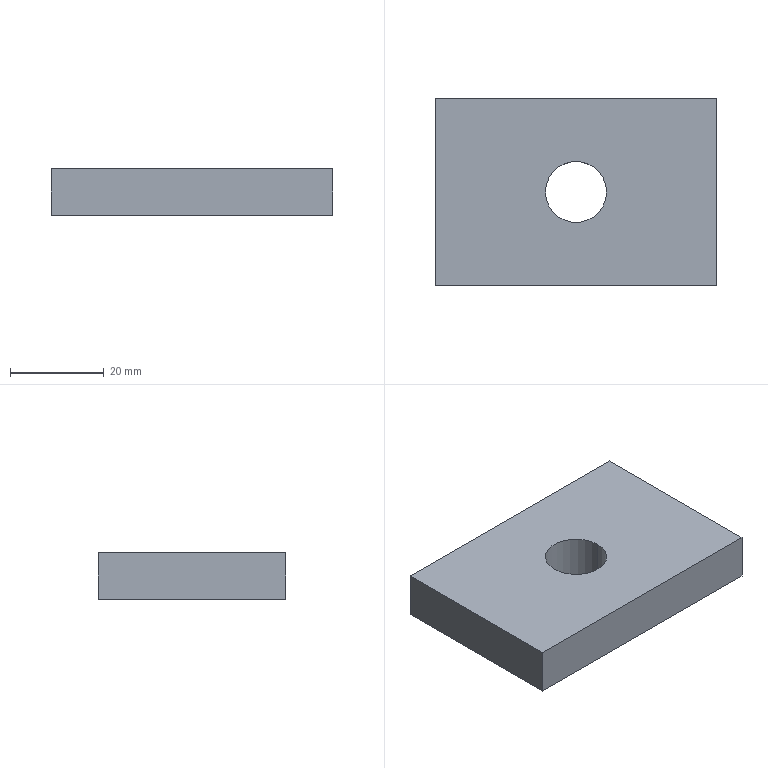Part | SolidWorks | features BaseBody 1 | 1 solid | 8 faces | box 60 x 40 x 10 mm | volume 22673 mm3 | plane 6 | cylinder 2 | commonest cylinder face diameters 13 x2
STEP:
#1=CARTESIAN_POINT('',(6.5,0.,0.));
#2=VERTEX_POINT('',#1);
#3=CARTESIAN_POINT('',(-6.5,0.,0.));
#4=VERTEX_POINT('',#3);
#5=CARTESIAN_POINT('',(0.,0.,0.));
#6=DIRECTION('',(0.,0.,-1.));
#7=DIRECTION('',(1.,0.,0.));
#8=AXIS2_PLACEMENT_3D('',#5,#6,#7);
#9=CIRCLE('',#8,6.5);
#10=EDGE_CURVE('',#2,#4,#9,.T.);
#11=ORIENTED_EDGE('',*,*,#10,.T.);
#12=CARTESIAN_POINT('',(-6.5,0.,10.));
#13=VERTEX_POINT('',#12);
#14=CARTESIAN_POINT('',(-6.5,0.,0.));
#15=DIRECTION('',(0.,0.,1.));
#16=VECTOR('',#15,1000.);
#17=LINE('',#14,#16);
#18=EDGE_CURVE('',#4,#13,#17,.T.);
#19=ORIENTED_EDGE('',*,*,#18,.T.);
#20=CARTESIAN_POINT('',(6.5,0.,10.));
#21=VERTEX_POINT('',#20);
#22=CARTESIAN_POINT('',(0.,0.,10.));
#23=DIRECTION('',(0.,0.,-1.));
#24=DIRECTION('',(1.,0.,0.));
#25=AXIS2_PLACEMENT_3D('',#22,#23,#24);
#26=CIRCLE('',#25,6.5);
#27=EDGE_CURVE('',#21,#13,#26,.T.);
#28=ORIENTED_EDGE('',*,*,#27,.F.);
#29=CARTESIAN_POINT('',(6.5,0.,0.));
#30=DIRECTION('',(0.,0.,1.));
#31=VECTOR('',#30,1000.);
#32=LINE('',#29,#31);
#33=EDGE_CURVE('',#2,#21,#32,.T.);
#34=ORIENTED_EDGE('',*,*,#33,.F.);
#35=EDGE_LOOP('',(#11,#19,#28,#34));
#36=FACE_OUTER_BOUND('',#35,.T.);
#37=CARTESIAN_POINT('',(0.,0.,0.));
#38=DIRECTION('',(0.,0.,1.));
#39=DIRECTION('',(1.,0.,0.));
#40=AXIS2_PLACEMENT_3D('',#37,#38,#39);
#41=CYLINDRICAL_SURFACE('',#40,6.5);
#42=ADVANCED_FACE('',(#36),#41,.F.);
#43=ORIENTED_EDGE('',*,*,#10,.F.);
#44=CARTESIAN_POINT('',(0.,0.,0.));
#45=DIRECTION('',(0.,0.,-1.));
#46=DIRECTION('',(1.,0.,0.));
#47=AXIS2_PLACEMENT_3D('',#44,#45,#46);
#48=CIRCLE('',#47,6.5);
#49=EDGE_CURVE('',#4,#2,#48,.T.);
#50=ORIENTED_EDGE('',*,*,#49,.F.);
#51=EDGE_LOOP('',(#43,#50));
#52=FACE_BOUND('',#51,.T.);
#53=CARTESIAN_POINT('',(30.,-20.,0.));
#54=VERTEX_POINT('',#53);
#55=CARTESIAN_POINT('',(30.,20.,0.));
#56=VERTEX_POINT('',#55);
#57=CARTESIAN_POINT('',(30.,0.,0.));
#58=DIRECTION('',(0.,1.,0.));
#59=VECTOR('',#58,1000.);
#60=LINE('',#57,#59);
#61=EDGE_CURVE('',#54,#56,#60,.T.);
#62=ORIENTED_EDGE('',*,*,#61,.F.);
#63=CARTESIAN_POINT('',(-30.,-20.,0.));
#64=VERTEX_POINT('',#63);
#65=CARTESIAN_POINT('',(0.,-20.,0.));
#66=DIRECTION('',(1.,0.,0.));
#67=VECTOR('',#66,1000.);
#68=LINE('',#65,#67);
#69=EDGE_CURVE('',#64,#54,#68,.T.);
#70=ORIENTED_EDGE('',*,*,#69,.F.);
#71=CARTESIAN_POINT('',(-30.,20.,0.));
#72=VERTEX_POINT('',#71);
#73=CARTESIAN_POINT('',(-30.,0.,0.));
#74=DIRECTION('',(0.,-1.,0.));
#75=VECTOR('',#74,1000.);
#76=LINE('',#73,#75);
#77=EDGE_CURVE('',#72,#64,#76,.T.);
#78=ORIENTED_EDGE('',*,*,#77,.F.);
#79=CARTESIAN_POINT('',(0.,20.,0.));
#80=DIRECTION('',(-1.,0.,0.));
#81=VECTOR('',#80,1000.);
#82=LINE('',#79,#81);
#83=EDGE_CURVE('',#56,#72,#82,.T.);
#84=ORIENTED_EDGE('',*,*,#83,.F.);
#85=EDGE_LOOP('',(#62,#70,#78,#84));
#86=FACE_OUTER_BOUND('',#85,.T.);
#87=CARTESIAN_POINT('',(0.,0.,0.));
#88=DIRECTION('',(0.,0.,1.));
#89=DIRECTION('',(1.,0.,0.));
#90=AXIS2_PLACEMENT_3D('',#87,#88,#89);
#91=PLANE('',#90);
#92=ADVANCED_FACE('',(#52,#86),#91,.F.);
#93=ORIENTED_EDGE('',*,*,#18,.F.);
#94=ORIENTED_EDGE('',*,*,#49,.T.);
#95=ORIENTED_EDGE('',*,*,#33,.T.);
#96=CARTESIAN_POINT('',(0.,0.,10.));
#97=DIRECTION('',(0.,0.,-1.));
#98=DIRECTION('',(1.,0.,0.));
#99=AXIS2_PLACEMENT_3D('',#96,#97,#98);
#100=CIRCLE('',#99,6.5);
#101=EDGE_CURVE('',#13,#21,#100,.T.);
#102=ORIENTED_EDGE('',*,*,#101,.F.);
#103=EDGE_LOOP('',(#93,#94,#95,#102));
#104=FACE_OUTER_BOUND('',#103,.T.);
#105=CARTESIAN_POINT('',(0.,0.,0.));
#106=DIRECTION('',(0.,0.,1.));
#107=DIRECTION('',(1.,0.,0.));
#108=AXIS2_PLACEMENT_3D('',#105,#106,#107);
#109=CYLINDRICAL_SURFACE('',#108,6.5);
#110=ADVANCED_FACE('',(#104),#109,.F.);
#111=ORIENTED_EDGE('',*,*,#83,.T.);
#112=CARTESIAN_POINT('',(-30.,20.,10.));
#113=VERTEX_POINT('',#112);
#114=CARTESIAN_POINT('',(-30.,20.,0.));
#115=DIRECTION('',(0.,0.,1.));
#116=VECTOR('',#115,1000.);
#117=LINE('',#114,#116);
#118=EDGE_CURVE('',#72,#113,#117,.T.);
#119=ORIENTED_EDGE('',*,*,#118,.T.);
#120=CARTESIAN_POINT('',(30.,20.,10.));
#121=VERTEX_POINT('',#120);
#122=CARTESIAN_POINT('',(-30.,20.,10.));
#123=DIRECTION('',(1.,0.,0.));
#124=VECTOR('',#123,1000.);
#125=LINE('',#122,#124);
#126=EDGE_CURVE('',#113,#121,#125,.T.);
#127=ORIENTED_EDGE('',*,*,#126,.T.);
#128=CARTESIAN_POINT('',(30.,20.,0.));
#129=DIRECTION('',(0.,0.,-1.));
#130=VECTOR('',#129,1000.);
#131=LINE('',#128,#130);
#132=EDGE_CURVE('',#121,#56,#131,.T.);
#133=ORIENTED_EDGE('',*,*,#132,.T.);
#134=EDGE_LOOP('',(#111,#119,#127,#133));
#135=FACE_OUTER_BOUND('',#134,.T.);
#136=CARTESIAN_POINT('',(-30.,20.,0.));
#137=DIRECTION('',(0.,1.,0.));
#138=DIRECTION('',(0.,0.,1.));
#139=AXIS2_PLACEMENT_3D('',#136,#137,#138);
#140=PLANE('',#139);
#141=ADVANCED_FACE('',(#135),#140,.T.);
#142=ORIENTED_EDGE('',*,*,#61,.T.);
#143=ORIENTED_EDGE('',*,*,#132,.F.);
#144=CARTESIAN_POINT('',(30.,-20.,10.));
#145=VERTEX_POINT('',#144);
#146=CARTESIAN_POINT('',(30.,20.,10.));
#147=DIRECTION('',(0.,-1.,0.));
#148=VECTOR('',#147,1000.);
#149=LINE('',#146,#148);
#150=EDGE_CURVE('',#121,#145,#149,.T.);
#151=ORIENTED_EDGE('',*,*,#150,.T.);
#152=CARTESIAN_POINT('',(30.,-20.,0.));
#153=DIRECTION('',(0.,0.,-1.));
#154=VECTOR('',#153,1000.);
#155=LINE('',#152,#154);
#156=EDGE_CURVE('',#145,#54,#155,.T.);
#157=ORIENTED_EDGE('',*,*,#156,.T.);
#158=EDGE_LOOP('',(#142,#143,#151,#157));
#159=FACE_OUTER_BOUND('',#158,.T.);
#160=CARTESIAN_POINT('',(30.,20.,0.));
#161=DIRECTION('',(1.,0.,0.));
#162=DIRECTION('',(0.,1.,0.));
#163=AXIS2_PLACEMENT_3D('',#160,#161,#162);
#164=PLANE('',#163);
#165=ADVANCED_FACE('',(#159),#164,.T.);
#166=ORIENTED_EDGE('',*,*,#69,.T.);
#167=ORIENTED_EDGE('',*,*,#156,.F.);
#168=CARTESIAN_POINT('',(-30.,-20.,10.));
#169=VERTEX_POINT('',#168);
#170=CARTESIAN_POINT('',(30.,-20.,10.));
#171=DIRECTION('',(-1.,0.,0.));
#172=VECTOR('',#171,1000.);
#173=LINE('',#170,#172);
#174=EDGE_CURVE('',#145,#169,#173,.T.);
#175=ORIENTED_EDGE('',*,*,#174,.T.);
#176=CARTESIAN_POINT('',(-30.,-20.,0.));
#177=DIRECTION('',(0.,0.,-1.));
#178=VECTOR('',#177,1000.);
#179=LINE('',#176,#178);
#180=EDGE_CURVE('',#169,#64,#179,.T.);
#181=ORIENTED_EDGE('',*,*,#180,.T.);
#182=EDGE_LOOP('',(#166,#167,#175,#181));
#183=FACE_OUTER_BOUND('',#182,.T.);
#184=CARTESIAN_POINT('',(30.,-20.,0.));
#185=DIRECTION('',(0.,-1.,0.));
#186=DIRECTION('',(1.,0.,0.));
#187=AXIS2_PLACEMENT_3D('',#184,#185,#186);
#188=PLANE('',#187);
#189=ADVANCED_FACE('',(#183),#188,.T.);
#190=ORIENTED_EDGE('',*,*,#77,.T.);
#191=ORIENTED_EDGE('',*,*,#180,.F.);
#192=CARTESIAN_POINT('',(-30.,-20.,10.));
#193=DIRECTION('',(0.,1.,0.));
#194=VECTOR('',#193,1000.);
#195=LINE('',#192,#194);
#196=EDGE_CURVE('',#169,#113,#195,.T.);
#197=ORIENTED_EDGE('',*,*,#196,.T.);
#198=ORIENTED_EDGE('',*,*,#118,.F.);
#199=EDGE_LOOP('',(#190,#191,#197,#198));
#200=FACE_OUTER_BOUND('',#199,.T.);
#201=CARTESIAN_POINT('',(-30.,-20.,0.));
#202=DIRECTION('',(-1.,0.,0.));
#203=DIRECTION('',(0.,-1.,0.));
#204=AXIS2_PLACEMENT_3D('',#201,#202,#203);
#205=PLANE('',#204);
#206=ADVANCED_FACE('',(#200),#205,.T.);
#207=ORIENTED_EDGE('',*,*,#27,.T.);
#208=ORIENTED_EDGE('',*,*,#101,.T.);
#209=EDGE_LOOP('',(#207,#208));
#210=FACE_BOUND('',#209,.T.);
#211=ORIENTED_EDGE('',*,*,#196,.F.);
#212=ORIENTED_EDGE('',*,*,#174,.F.);
#213=ORIENTED_EDGE('',*,*,#150,.F.);
#214=ORIENTED_EDGE('',*,*,#126,.F.);
#215=EDGE_LOOP('',(#211,#212,#213,#214));
#216=FACE_OUTER_BOUND('',#215,.T.);
#217=CARTESIAN_POINT('',(0.,0.,10.));
#218=DIRECTION('',(0.,0.,1.));
#219=DIRECTION('',(1.,0.,0.));
#220=AXIS2_PLACEMENT_3D('',#217,#218,#219);
#221=PLANE('',#220);
#222=ADVANCED_FACE('',(#210,#216),#221,.T.);
#223=CLOSED_SHELL('',(#42,#92,#110,#141,#165,#189,#206,#222));
#224=MANIFOLD_SOLID_BREP('',#223);
#225=CARTESIAN_POINT('',(0.,0.,0.));
#226=DIRECTION('',(0.,0.,1.));
#227=DIRECTION('',(1.,0.,0.));
#228=AXIS2_PLACEMENT_3D('',#225,#226,#227);
#229=(LENGTH_UNIT()NAMED_UNIT(*)SI_UNIT(.MILLI.,.METRE.));
#230=UNCERTAINTY_MEASURE_WITH_UNIT(LENGTH_MEASURE(0.00001),#229,'','');
#231=(NAMED_UNIT(*)PLANE_ANGLE_UNIT()SI_UNIT($,.RADIAN.));
#232=(NAMED_UNIT(*)SI_UNIT($,.STERADIAN.)SOLID_ANGLE_UNIT());
#233=(GEOMETRIC_REPRESENTATION_CONTEXT(3)GLOBAL_UNCERTAINTY_ASSIGNED_CONTEXT((#230))GLOBAL_UNIT_ASSIGNED_CONTEXT((#229,#231,#232))REPRESENTATION_CONTEXT('',''));
#234=ADVANCED_BREP_SHAPE_REPRESENTATION('',(#224,#228),#233);